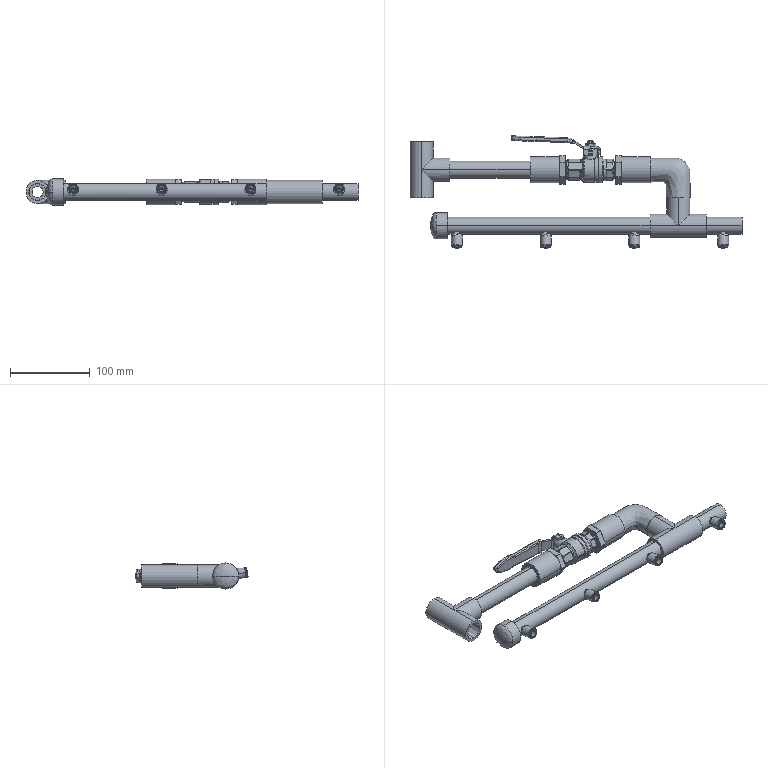Part | SolidWorks | 19 solids | 1135 faces | box 415.26 x 140.383 x 32.766 mm | volume 299661 mm3 | cylinder 284 | spline 275 | plane 266 | cone 207 | sphere 52 | torus 51 | commonest cylinder face diameters 0.635 x62 7 x27 13.868 x24 1.27 x20 2.54 x17 8 x16